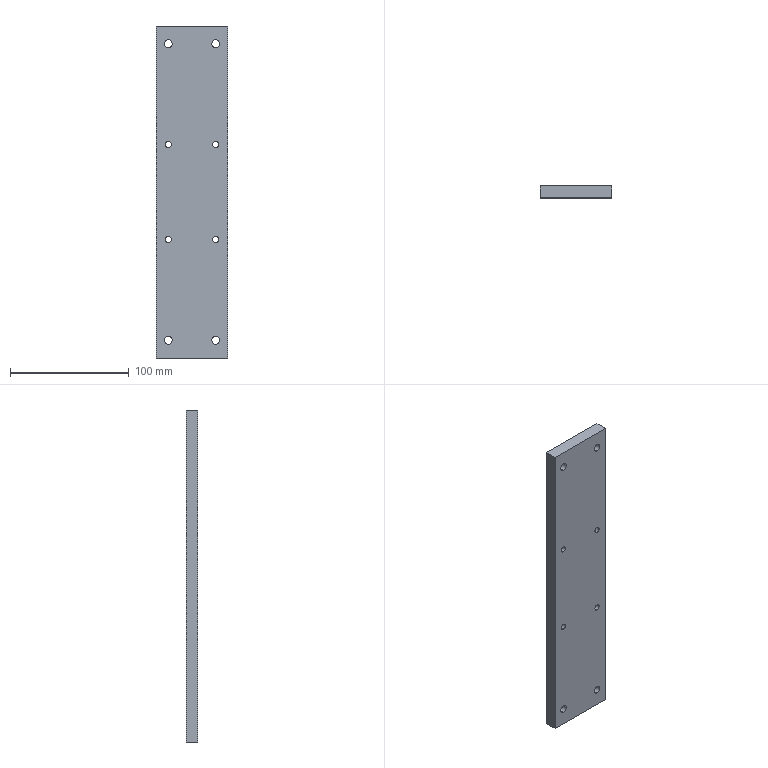Part | STEP file | Movable tube support mount | 1 solid | 22 faces | box 60 x 10 x 280 mm | volume 165846 mm3 | cylinder 16 | plane 6 | commonest cylinder face diameters 5 x8 6.6 x8